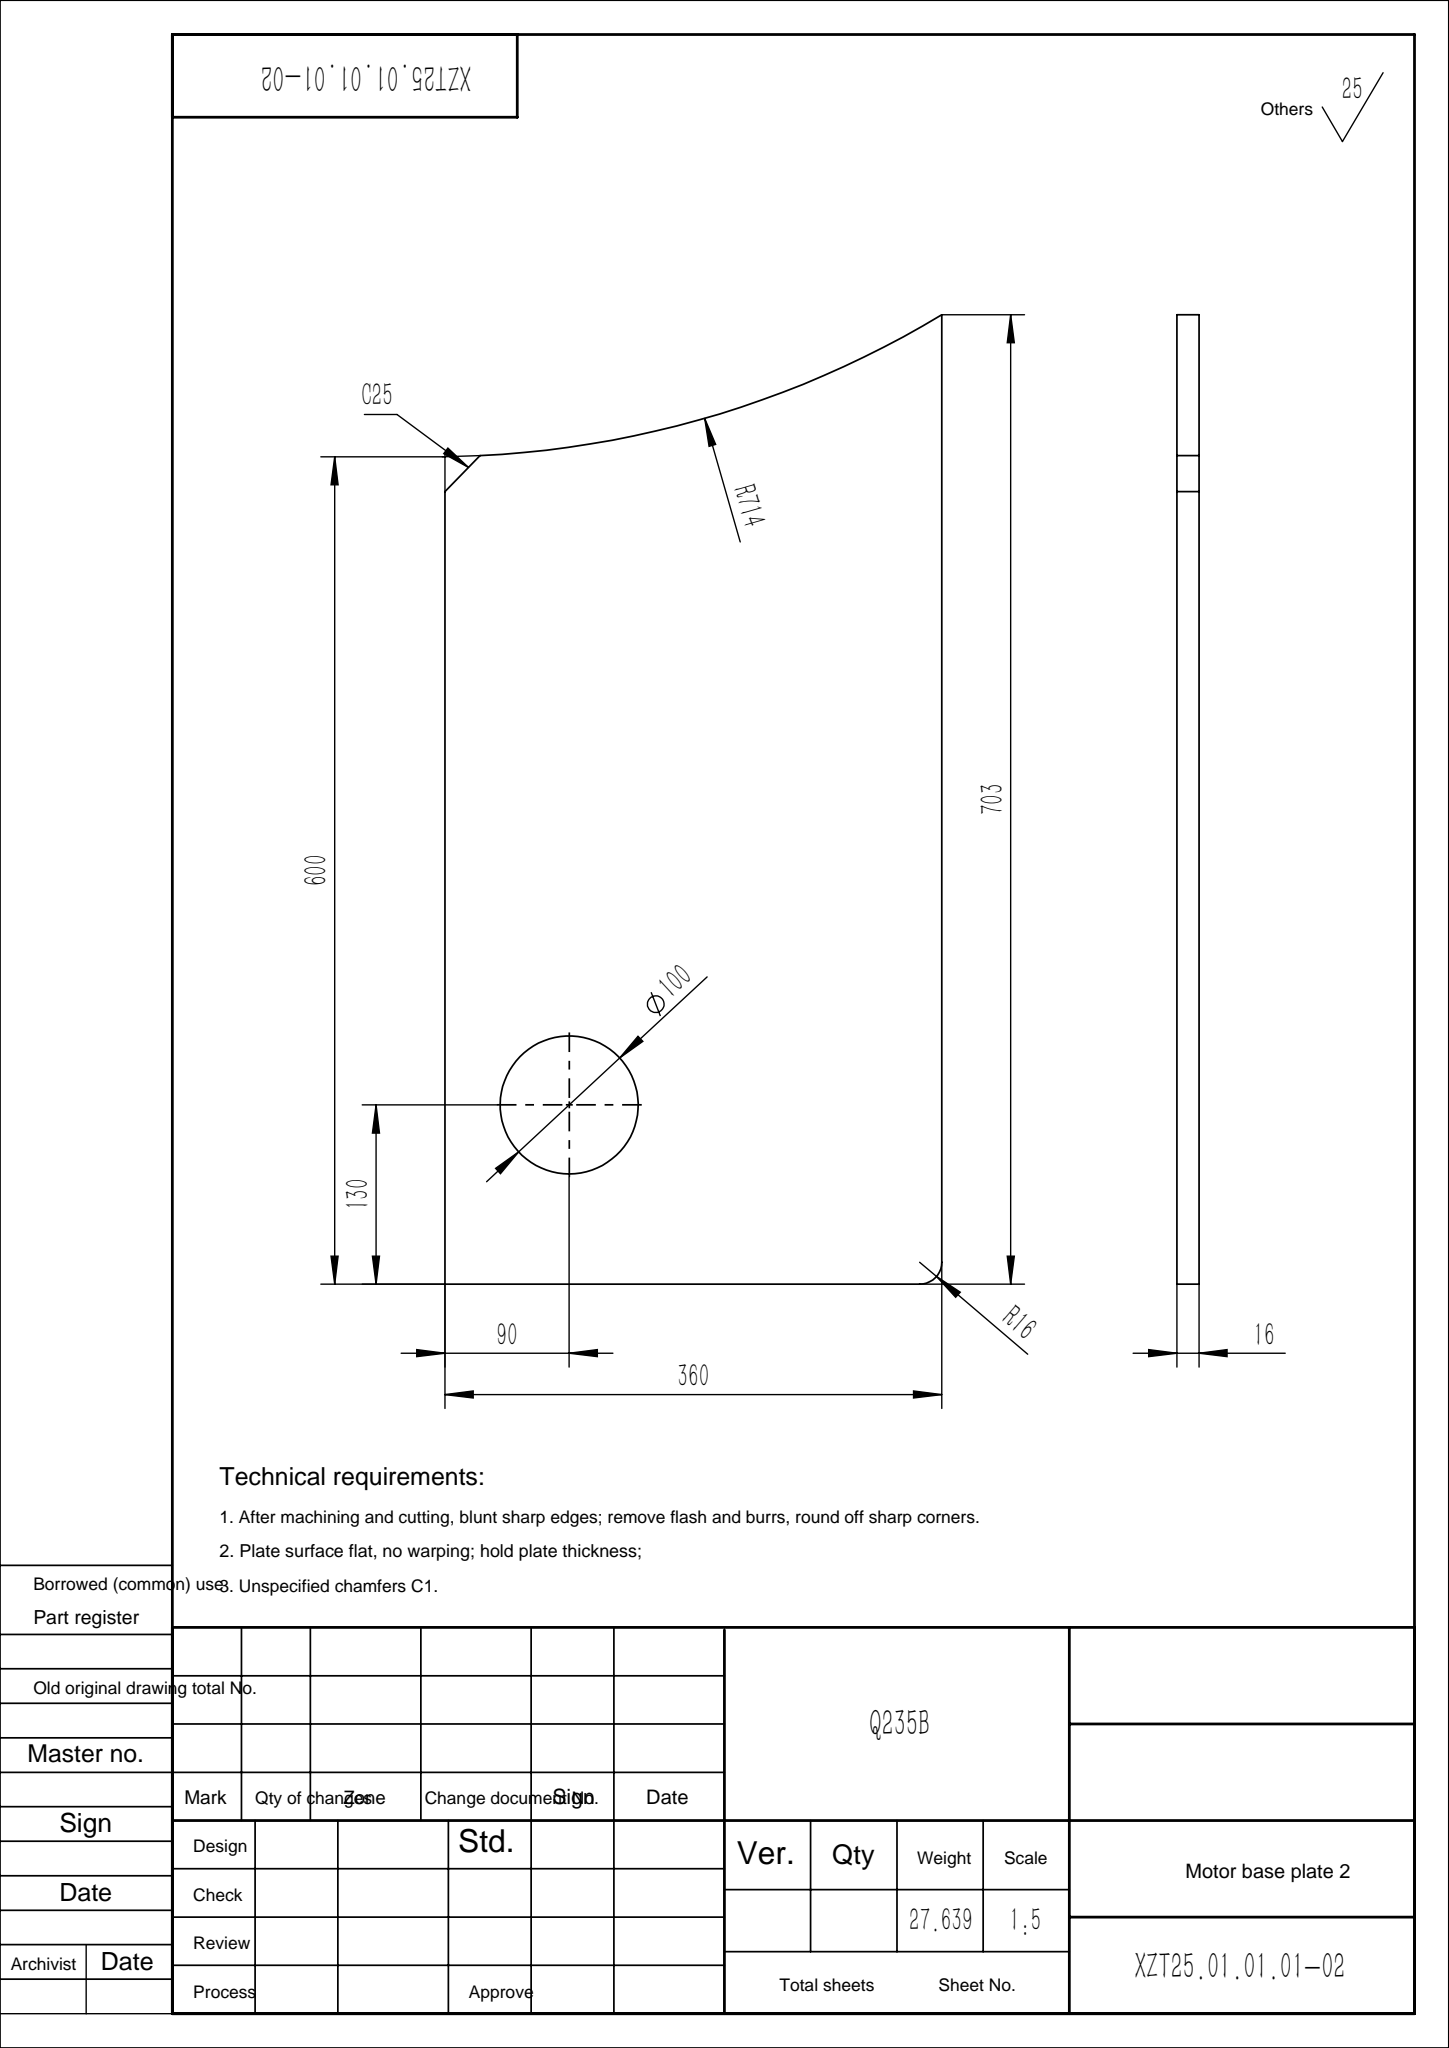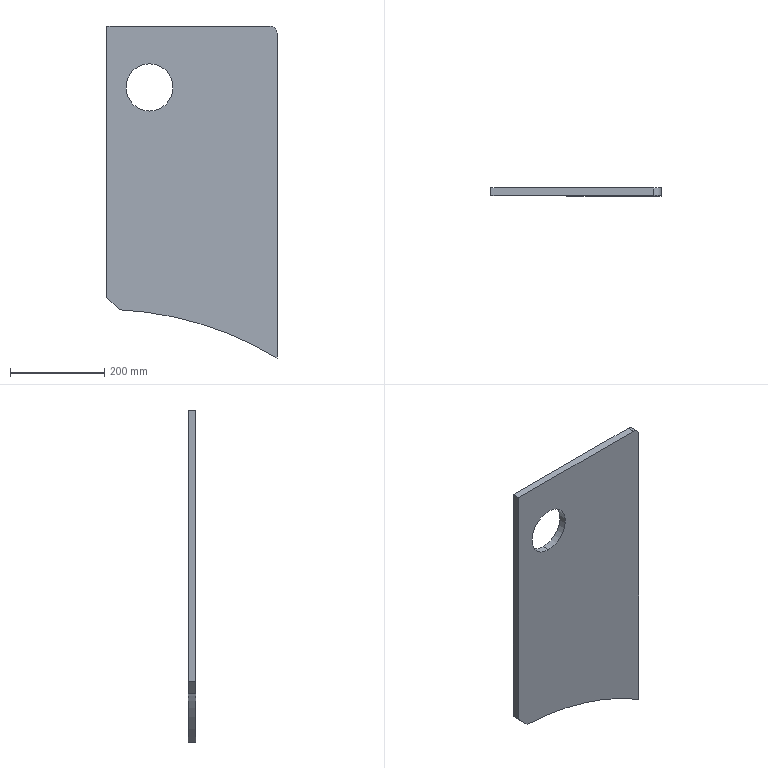Part | SolidWorks | features Chamfer 1, Extrusion 1, Fillet 1 | 1 solid | 10 faces | box 360 x 16 x 703 mm | volume 3520829 mm3 | plane 6 | cylinder 4 | commonest cylinder face diameters 100 x2 32 x1 1428 x1
STEP:
#1=CARTESIAN_POINT('',(90.,8.,-180.));
#2=VERTEX_POINT('',#1);
#3=CARTESIAN_POINT('',(90.,8.,-80.));
#4=VERTEX_POINT('',#3);
#5=CARTESIAN_POINT('',(90.,8.,-130.));
#6=DIRECTION('',(0.,1.,0.));
#7=DIRECTION('',(0.,0.,1.));
#8=AXIS2_PLACEMENT_3D('',#5,#6,#7);
#9=CIRCLE('',#8,50.);
#10=EDGE_CURVE('',#2,#4,#9,.T.);
#11=ORIENTED_EDGE('',*,*,#10,.T.);
#12=CARTESIAN_POINT('',(90.,-8.,-80.));
#13=VERTEX_POINT('',#12);
#14=CARTESIAN_POINT('',(90.,8.,-80.));
#15=DIRECTION('',(0.,-1.,0.));
#16=VECTOR('',#15,1000.);
#17=LINE('',#14,#16);
#18=EDGE_CURVE('',#4,#13,#17,.T.);
#19=ORIENTED_EDGE('',*,*,#18,.T.);
#20=CARTESIAN_POINT('',(90.,-8.,-180.));
#21=VERTEX_POINT('',#20);
#22=CARTESIAN_POINT('',(90.,-8.,-130.));
#23=DIRECTION('',(0.,1.,0.));
#24=DIRECTION('',(0.,0.,1.));
#25=AXIS2_PLACEMENT_3D('',#22,#23,#24);
#26=CIRCLE('',#25,50.);
#27=EDGE_CURVE('',#21,#13,#26,.T.);
#28=ORIENTED_EDGE('',*,*,#27,.F.);
#29=CARTESIAN_POINT('',(90.,8.,-180.));
#30=DIRECTION('',(0.,-1.,0.));
#31=VECTOR('',#30,1000.);
#32=LINE('',#29,#31);
#33=EDGE_CURVE('',#2,#21,#32,.T.);
#34=ORIENTED_EDGE('',*,*,#33,.F.);
#35=EDGE_LOOP('',(#11,#19,#28,#34));
#36=FACE_OUTER_BOUND('',#35,.T.);
#37=CARTESIAN_POINT('',(90.,8.,-130.));
#38=DIRECTION('',(0.,-1.,0.));
#39=DIRECTION('',(0.,0.,-1.));
#40=AXIS2_PLACEMENT_3D('',#37,#38,#39);
#41=CYLINDRICAL_SURFACE('',#40,50.);
#42=ADVANCED_FACE('',(#36),#41,.F.);
#43=CARTESIAN_POINT('',(0.,8.,0.));
#44=VERTEX_POINT('',#43);
#45=CARTESIAN_POINT('',(344.,8.,0.));
#46=VERTEX_POINT('',#45);
#47=CARTESIAN_POINT('',(0.,8.,0.));
#48=DIRECTION('',(1.,0.,0.));
#49=VECTOR('',#48,1000.);
#50=LINE('',#47,#49);
#51=EDGE_CURVE('',#44,#46,#50,.T.);
#52=ORIENTED_EDGE('',*,*,#51,.T.);
#53=CARTESIAN_POINT('',(360.,8.,-16.));
#54=VERTEX_POINT('',#53);
#55=CARTESIAN_POINT('',(344.,8.,-16.));
#56=DIRECTION('',(0.,1.,0.));
#57=DIRECTION('',(0.,0.,1.));
#58=AXIS2_PLACEMENT_3D('',#55,#56,#57);
#59=CIRCLE('',#58,16.);
#60=EDGE_CURVE('',#46,#54,#59,.T.);
#61=ORIENTED_EDGE('',*,*,#60,.T.);
#62=CARTESIAN_POINT('',(360.,8.,-703.));
#63=VERTEX_POINT('',#62);
#64=CARTESIAN_POINT('',(360.,8.,0.));
#65=DIRECTION('',(0.,0.,-1.));
#66=VECTOR('',#65,1000.);
#67=LINE('',#64,#66);
#68=EDGE_CURVE('',#54,#63,#67,.T.);
#69=ORIENTED_EDGE('',*,*,#68,.T.);
#70=CARTESIAN_POINT('',(25.446,8.,-600.794));
#71=VERTEX_POINT('',#70);
#72=CARTESIAN_POINT('',(-9.53,8.,-1313.936));
#73=DIRECTION('',(0.,-1.,0.));
#74=DIRECTION('',(0.,0.,1.));
#75=AXIS2_PLACEMENT_3D('',#72,#73,#74);
#76=CIRCLE('',#75,714.);
#77=EDGE_CURVE('',#63,#71,#76,.T.);
#78=ORIENTED_EDGE('',*,*,#77,.T.);
#79=CARTESIAN_POINT('',(0.,8.,-574.659));
#80=VERTEX_POINT('',#79);
#81=CARTESIAN_POINT('',(364.869,8.,-949.401));
#82=DIRECTION('',(-0.6976,0.,0.7165));
#83=VECTOR('',#82,1000.);
#84=LINE('',#81,#83);
#85=EDGE_CURVE('',#71,#80,#84,.T.);
#86=ORIENTED_EDGE('',*,*,#85,.T.);
#87=CARTESIAN_POINT('',(0.,8.,0.));
#88=DIRECTION('',(0.,0.,1.));
#89=VECTOR('',#88,1000.);
#90=LINE('',#87,#89);
#91=EDGE_CURVE('',#80,#44,#90,.T.);
#92=ORIENTED_EDGE('',*,*,#91,.T.);
#93=EDGE_LOOP('',(#52,#61,#69,#78,#86,#92));
#94=FACE_OUTER_BOUND('',#93,.T.);
#95=ORIENTED_EDGE('',*,*,#10,.F.);
#96=CARTESIAN_POINT('',(90.,8.,-130.));
#97=DIRECTION('',(0.,1.,0.));
#98=DIRECTION('',(0.,0.,1.));
#99=AXIS2_PLACEMENT_3D('',#96,#97,#98);
#100=CIRCLE('',#99,50.);
#101=EDGE_CURVE('',#4,#2,#100,.T.);
#102=ORIENTED_EDGE('',*,*,#101,.F.);
#103=EDGE_LOOP('',(#95,#102));
#104=FACE_BOUND('',#103,.T.);
#105=CARTESIAN_POINT('',(-9.53,8.,-1313.936));
#106=DIRECTION('',(0.,1.,0.));
#107=DIRECTION('',(0.,0.,1.));
#108=AXIS2_PLACEMENT_3D('',#105,#106,#107);
#109=PLANE('',#108);
#110=ADVANCED_FACE('',(#94,#104),#109,.T.);
#111=CARTESIAN_POINT('',(360.,-8.,-16.));
#112=VERTEX_POINT('',#111);
#113=CARTESIAN_POINT('',(360.,-8.,-703.));
#114=VERTEX_POINT('',#113);
#115=CARTESIAN_POINT('',(360.,-8.,0.));
#116=DIRECTION('',(0.,0.,-1.));
#117=VECTOR('',#116,1000.);
#118=LINE('',#115,#117);
#119=EDGE_CURVE('',#112,#114,#118,.T.);
#120=ORIENTED_EDGE('',*,*,#119,.F.);
#121=CARTESIAN_POINT('',(344.,-8.,0.));
#122=VERTEX_POINT('',#121);
#123=CARTESIAN_POINT('',(344.,-8.,-16.));
#124=DIRECTION('',(0.,-1.,0.));
#125=DIRECTION('',(0.,0.,1.));
#126=AXIS2_PLACEMENT_3D('',#123,#124,#125);
#127=CIRCLE('',#126,16.);
#128=EDGE_CURVE('',#112,#122,#127,.T.);
#129=ORIENTED_EDGE('',*,*,#128,.T.);
#130=CARTESIAN_POINT('',(0.,-8.,0.));
#131=VERTEX_POINT('',#130);
#132=CARTESIAN_POINT('',(0.,-8.,0.));
#133=DIRECTION('',(1.,0.,0.));
#134=VECTOR('',#133,1000.);
#135=LINE('',#132,#134);
#136=EDGE_CURVE('',#131,#122,#135,.T.);
#137=ORIENTED_EDGE('',*,*,#136,.F.);
#138=CARTESIAN_POINT('',(0.,-8.,-574.659));
#139=VERTEX_POINT('',#138);
#140=CARTESIAN_POINT('',(0.,-8.,0.));
#141=DIRECTION('',(0.,0.,1.));
#142=VECTOR('',#141,1000.);
#143=LINE('',#140,#142);
#144=EDGE_CURVE('',#139,#131,#143,.T.);
#145=ORIENTED_EDGE('',*,*,#144,.F.);
#146=CARTESIAN_POINT('',(25.446,-8.,-600.794));
#147=VERTEX_POINT('',#146);
#148=CARTESIAN_POINT('',(0.,-8.,-574.659));
#149=DIRECTION('',(0.6976,0.,-0.7165));
#150=VECTOR('',#149,1000.);
#151=LINE('',#148,#150);
#152=EDGE_CURVE('',#139,#147,#151,.T.);
#153=ORIENTED_EDGE('',*,*,#152,.T.);
#154=CARTESIAN_POINT('',(-9.53,-8.,-1313.936));
#155=DIRECTION('',(0.,-1.,0.));
#156=DIRECTION('',(0.,0.,1.));
#157=AXIS2_PLACEMENT_3D('',#154,#155,#156);
#158=CIRCLE('',#157,714.);
#159=EDGE_CURVE('',#114,#147,#158,.T.);
#160=ORIENTED_EDGE('',*,*,#159,.F.);
#161=EDGE_LOOP('',(#120,#129,#137,#145,#153,#160));
#162=FACE_OUTER_BOUND('',#161,.T.);
#163=ORIENTED_EDGE('',*,*,#27,.T.);
#164=CARTESIAN_POINT('',(90.,-8.,-130.));
#165=DIRECTION('',(0.,1.,0.));
#166=DIRECTION('',(0.,0.,1.));
#167=AXIS2_PLACEMENT_3D('',#164,#165,#166);
#168=CIRCLE('',#167,50.);
#169=EDGE_CURVE('',#13,#21,#168,.T.);
#170=ORIENTED_EDGE('',*,*,#169,.T.);
#171=EDGE_LOOP('',(#163,#170));
#172=FACE_BOUND('',#171,.T.);
#173=CARTESIAN_POINT('',(-9.53,-8.,-1313.936));
#174=DIRECTION('',(0.,1.,0.));
#175=DIRECTION('',(0.,0.,1.));
#176=AXIS2_PLACEMENT_3D('',#173,#174,#175);
#177=PLANE('',#176);
#178=ADVANCED_FACE('',(#162,#172),#177,.F.);
#179=ORIENTED_EDGE('',*,*,#136,.T.);
#180=CARTESIAN_POINT('',(344.,8.,0.));
#181=DIRECTION('',(0.,1.,0.));
#182=VECTOR('',#181,1000.);
#183=LINE('',#180,#182);
#184=EDGE_CURVE('',#122,#46,#183,.T.);
#185=ORIENTED_EDGE('',*,*,#184,.T.);
#186=ORIENTED_EDGE('',*,*,#51,.F.);
#187=CARTESIAN_POINT('',(0.,8.,0.));
#188=DIRECTION('',(0.,-1.,0.));
#189=VECTOR('',#188,1000.);
#190=LINE('',#187,#189);
#191=EDGE_CURVE('',#44,#131,#190,.T.);
#192=ORIENTED_EDGE('',*,*,#191,.T.);
#193=EDGE_LOOP('',(#179,#185,#186,#192));
#194=FACE_OUTER_BOUND('',#193,.T.);
#195=CARTESIAN_POINT('',(0.,8.,0.));
#196=DIRECTION('',(0.,0.,-1.));
#197=DIRECTION('',(-1.,0.,0.));
#198=AXIS2_PLACEMENT_3D('',#195,#196,#197);
#199=PLANE('',#198);
#200=ADVANCED_FACE('',(#194),#199,.F.);
#201=ORIENTED_EDGE('',*,*,#68,.F.);
#202=CARTESIAN_POINT('',(360.,8.,-16.));
#203=DIRECTION('',(0.,-1.,0.));
#204=VECTOR('',#203,1000.);
#205=LINE('',#202,#204);
#206=EDGE_CURVE('',#54,#112,#205,.T.);
#207=ORIENTED_EDGE('',*,*,#206,.T.);
#208=ORIENTED_EDGE('',*,*,#119,.T.);
#209=CARTESIAN_POINT('',(360.,8.,-703.));
#210=DIRECTION('',(0.,-1.,0.));
#211=VECTOR('',#210,1000.);
#212=LINE('',#209,#211);
#213=EDGE_CURVE('',#63,#114,#212,.T.);
#214=ORIENTED_EDGE('',*,*,#213,.F.);
#215=EDGE_LOOP('',(#201,#207,#208,#214));
#216=FACE_OUTER_BOUND('',#215,.T.);
#217=CARTESIAN_POINT('',(360.,8.,0.));
#218=DIRECTION('',(-1.,0.,0.));
#219=DIRECTION('',(0.,0.,1.));
#220=AXIS2_PLACEMENT_3D('',#217,#218,#219);
#221=PLANE('',#220);
#222=ADVANCED_FACE('',(#216),#221,.F.);
#223=ORIENTED_EDGE('',*,*,#159,.T.);
#224=CARTESIAN_POINT('',(25.446,8.,-600.794));
#225=DIRECTION('',(0.,1.,0.));
#226=VECTOR('',#225,1000.);
#227=LINE('',#224,#226);
#228=EDGE_CURVE('',#147,#71,#227,.T.);
#229=ORIENTED_EDGE('',*,*,#228,.T.);
#230=ORIENTED_EDGE('',*,*,#77,.F.);
#231=ORIENTED_EDGE('',*,*,#213,.T.);
#232=EDGE_LOOP('',(#223,#229,#230,#231));
#233=FACE_OUTER_BOUND('',#232,.T.);
#234=CARTESIAN_POINT('',(-9.53,8.,-1313.936));
#235=DIRECTION('',(0.,-1.,0.));
#236=DIRECTION('',(0.,0.,-1.));
#237=AXIS2_PLACEMENT_3D('',#234,#235,#236);
#238=CYLINDRICAL_SURFACE('',#237,714.);
#239=ADVANCED_FACE('',(#233),#238,.F.);
#240=ORIENTED_EDGE('',*,*,#91,.F.);
#241=CARTESIAN_POINT('',(0.,8.,-574.659));
#242=DIRECTION('',(0.,-1.,0.));
#243=VECTOR('',#242,1000.);
#244=LINE('',#241,#243);
#245=EDGE_CURVE('',#80,#139,#244,.T.);
#246=ORIENTED_EDGE('',*,*,#245,.T.);
#247=ORIENTED_EDGE('',*,*,#144,.T.);
#248=ORIENTED_EDGE('',*,*,#191,.F.);
#249=EDGE_LOOP('',(#240,#246,#247,#248));
#250=FACE_OUTER_BOUND('',#249,.T.);
#251=CARTESIAN_POINT('',(0.,8.,0.));
#252=DIRECTION('',(1.,0.,0.));
#253=DIRECTION('',(0.,0.,-1.));
#254=AXIS2_PLACEMENT_3D('',#251,#252,#253);
#255=PLANE('',#254);
#256=ADVANCED_FACE('',(#250),#255,.F.);
#257=ORIENTED_EDGE('',*,*,#18,.F.);
#258=ORIENTED_EDGE('',*,*,#101,.T.);
#259=ORIENTED_EDGE('',*,*,#33,.T.);
#260=ORIENTED_EDGE('',*,*,#169,.F.);
#261=EDGE_LOOP('',(#257,#258,#259,#260));
#262=FACE_OUTER_BOUND('',#261,.T.);
#263=CARTESIAN_POINT('',(90.,8.,-130.));
#264=DIRECTION('',(0.,-1.,0.));
#265=DIRECTION('',(0.,0.,-1.));
#266=AXIS2_PLACEMENT_3D('',#263,#264,#265);
#267=CYLINDRICAL_SURFACE('',#266,50.);
#268=ADVANCED_FACE('',(#262),#267,.F.);
#269=ORIENTED_EDGE('',*,*,#85,.F.);
#270=ORIENTED_EDGE('',*,*,#228,.F.);
#271=ORIENTED_EDGE('',*,*,#152,.F.);
#272=ORIENTED_EDGE('',*,*,#245,.F.);
#273=EDGE_LOOP('',(#269,#270,#271,#272));
#274=FACE_OUTER_BOUND('',#273,.T.);
#275=CARTESIAN_POINT('',(0.,8.,-574.659));
#276=DIRECTION('',(0.7165,0.,0.6976));
#277=DIRECTION('',(0.,-1.,0.));
#278=AXIS2_PLACEMENT_3D('',#275,#276,#277);
#279=PLANE('',#278);
#280=ADVANCED_FACE('',(#274),#279,.F.);
#281=ORIENTED_EDGE('',*,*,#60,.F.);
#282=ORIENTED_EDGE('',*,*,#184,.F.);
#283=ORIENTED_EDGE('',*,*,#128,.F.);
#284=ORIENTED_EDGE('',*,*,#206,.F.);
#285=EDGE_LOOP('',(#281,#282,#283,#284));
#286=FACE_OUTER_BOUND('',#285,.T.);
#287=CARTESIAN_POINT('',(344.,8.,-16.));
#288=DIRECTION('',(0.,-1.,0.));
#289=DIRECTION('',(0.,0.,-1.));
#290=AXIS2_PLACEMENT_3D('',#287,#288,#289);
#291=CYLINDRICAL_SURFACE('',#290,16.);
#292=ADVANCED_FACE('',(#286),#291,.T.);
#293=CLOSED_SHELL('',(#42,#110,#178,#200,#222,#239,#256,#268,#280,#292));
#294=MANIFOLD_SOLID_BREP('',#293);
#295=CARTESIAN_POINT('',(0.,0.,0.));
#296=DIRECTION('',(0.,0.,1.));
#297=DIRECTION('',(1.,0.,0.));
#298=AXIS2_PLACEMENT_3D('',#295,#296,#297);
#299=(LENGTH_UNIT()NAMED_UNIT(*)SI_UNIT(.MILLI.,.METRE.));
#300=UNCERTAINTY_MEASURE_WITH_UNIT(LENGTH_MEASURE(0.00001),#299,'','');
#301=(NAMED_UNIT(*)PLANE_ANGLE_UNIT()SI_UNIT($,.RADIAN.));
#302=(NAMED_UNIT(*)SI_UNIT($,.STERADIAN.)SOLID_ANGLE_UNIT());
#303=(GEOMETRIC_REPRESENTATION_CONTEXT(3)GLOBAL_UNCERTAINTY_ASSIGNED_CONTEXT((#300))GLOBAL_UNIT_ASSIGNED_CONTEXT((#299,#301,#302))REPRESENTATION_CONTEXT('',''));
#304=ADVANCED_BREP_SHAPE_REPRESENTATION('',(#294,#298),#303);